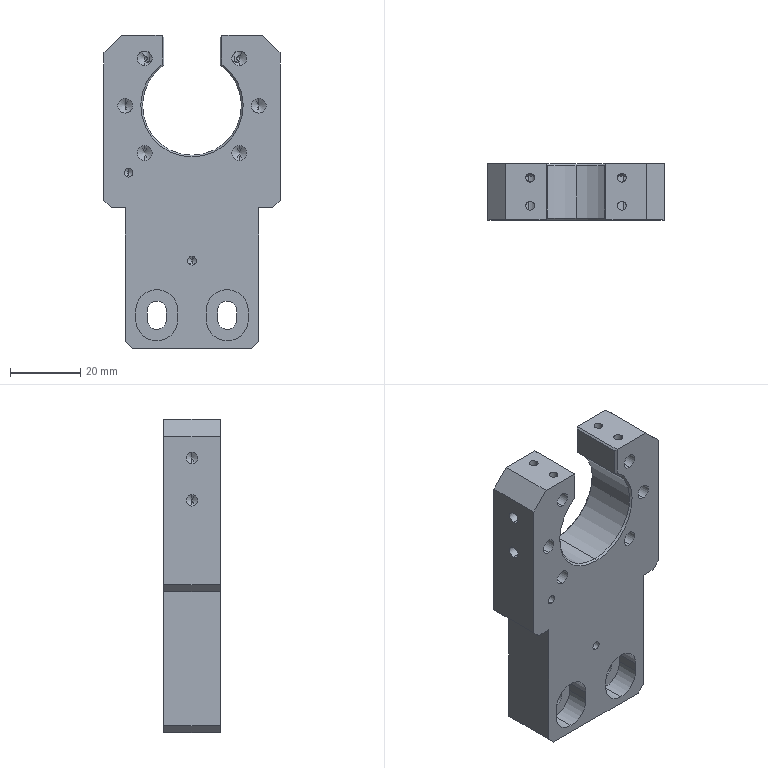Part | NX | features BREP 1 | 1 solid | 112 faces | box 50 x 16 x 89 mm | volume 47156 mm3 | cylinder 46 | plane 35 | cone 31 | commonest cylinder face diameters 2.5 x12 4.2 x12 3.3 x8 5.5 x6 12 x6 28.1 x2